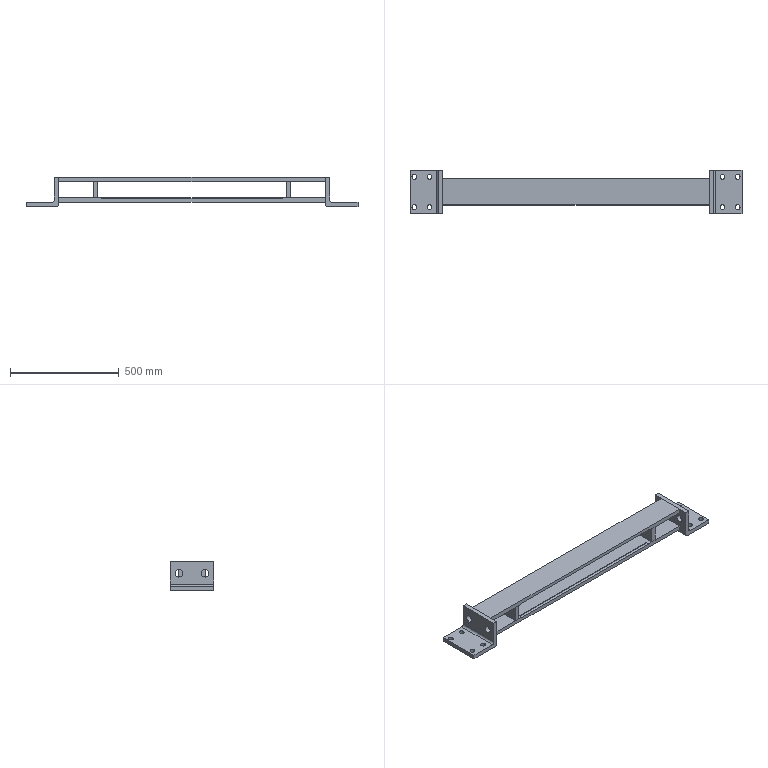Part | SolidWorks | features ICE 6, Fillet 2, Extrusion 1, HoleWzd 1, MirrorSolid 1, WeldmentFeature 1 | 6 solids | 84 faces | box 1530 x 200 x 135 mm | volume 8097209 mm3 | plane 52 | cylinder 32 | commonest cylinder face diameters 22 x16 20 x8 35 x8